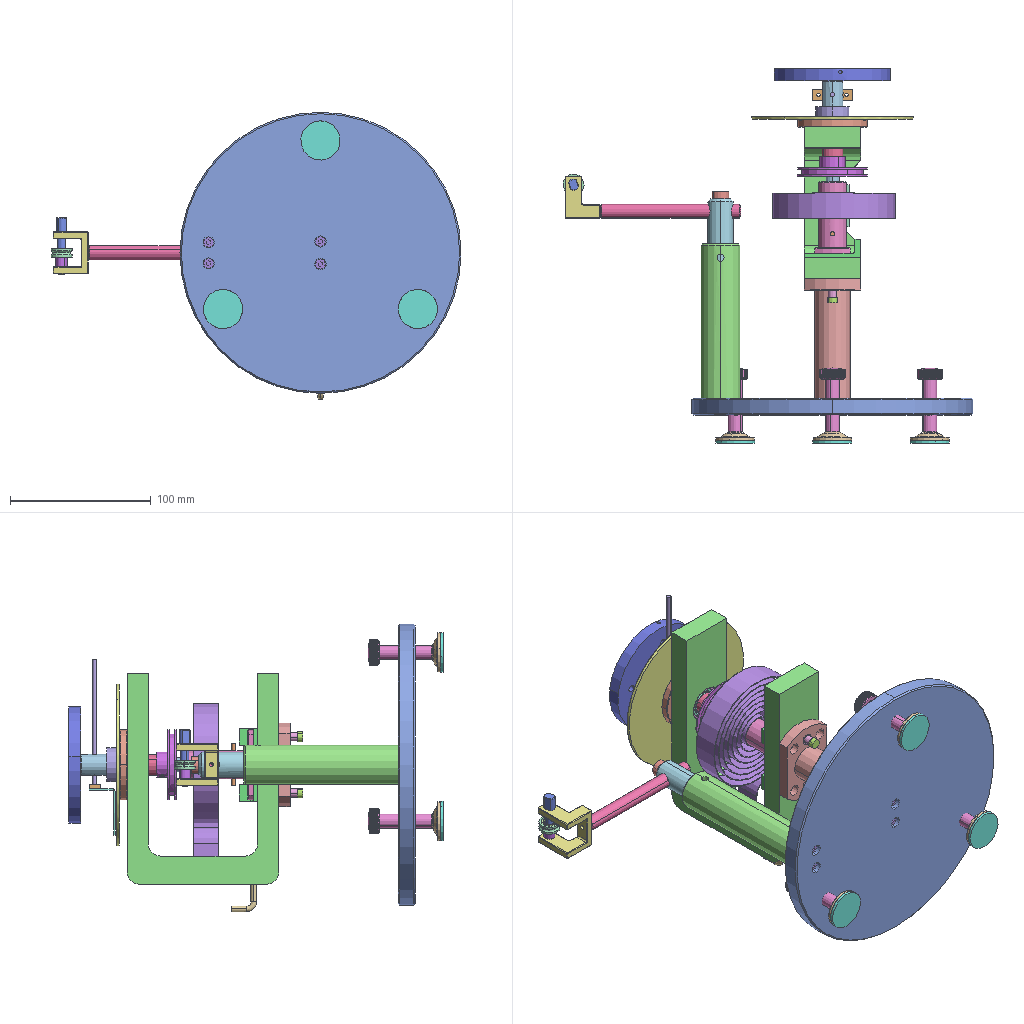Assembly | SolidWorks | 53 different items | 72 placed | box 292 x 266 x 204 mm
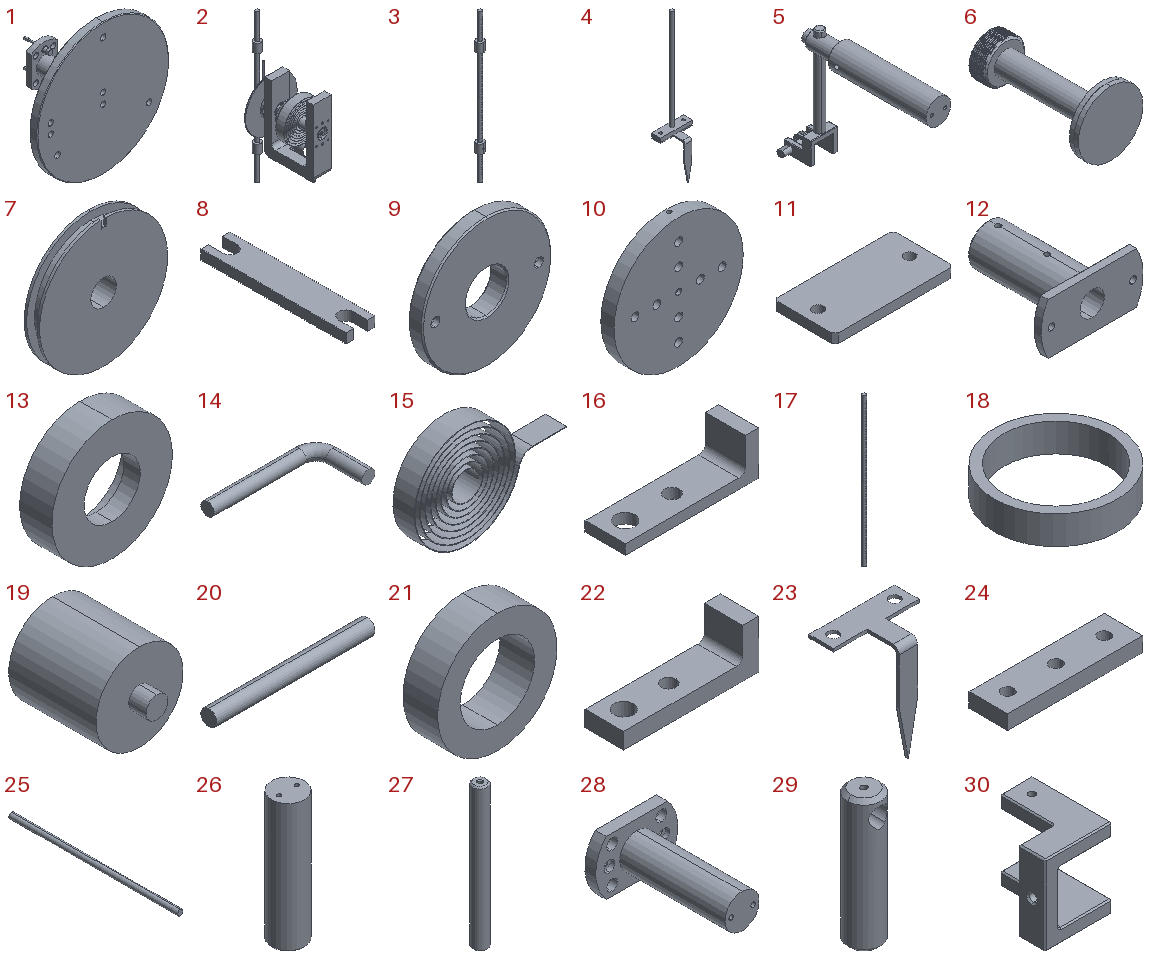Parts list (item | name | quantity | parent item | size | volume | features):
1 | (subassembly) | x1 | - | 200 x 119 x 200 mm | 427513 mm3 | -
2 | (subassembly) | x1 | - | 115 x 153 x 330 mm | 328755 mm3 | features CompositeCurve 2
3 | (subassembly) | x1 | in 2 | 16 x 16 x 330 mm | 22461 mm3 | features MirrorCompFeat 1, ReferencePattern 1
4 | (subassembly) | x1 | in 2 | 28 x 18.5 x 125 mm | 1686 mm3 | -
5 | (subassembly) | x1 | - | 40.5 x 159.5 x 126.5 mm | 84621 mm3 | -
6 | (subassembly) | x3 | - | 28 x 53.48 x 28 mm | 7166 mm3 | -
7 | - | x1 | in 2 | 50 x 14 x 50 mm | 10920 mm3 | features 3DProfileFeature 1, HoleWzd 1, ICE 1, Revolution 1
8 | - | x1 | in 2 | 6 x 30 x 2 mm | 309.863 mm3 | features Extrusion 1
9 | - | x1 | in 2 | 50 x 7 x 50 mm | 9665 mm3 | features 3DProfileFeature 1, Chamfer 1, HoleWzd 1, Revolution 1
10 | - | x1 | in 2 | 83 x 8.5 x 83 mm | 20251 mm3 | features 3DProfileFeature 1, Chamfer 1, HoleWzd 1, ICE 1, Revolution 1
11 | - | x1 | in 2 | 39 x 20 x 3 mm | 2276 mm3 | features Chamfer 1, Extrusion 1
12 | - | x1 | in 2 | 50 x 51 x 25 mm | 13586 mm3 | features 3DProfileFeature 2, HoleWzd 2, ICE 2, Chamfer 1, Revolution 1
13 | - | x1 | in 2 | 15 x 4 x 15 mm | 456.709 mm3 | features Revolution 1
14 | - | x1 | in 2 | 35 x 18 x 4 mm | 588.784 mm3 | features Sweep 1
15 | - | x1 | in 2 | 128.799 x 18 x 87.599 mm | 12839 mm3 | features Helix 1, Sweep 1
16 | - | x2 | in 2 | 40 x 12 x 13 mm | 1798 mm3 | features Extrusion 1, Fillet 1, ICE 1
17 | - | x1 | in 3 | 8 x 8 x 330 mm | 16519 mm3 | features ICE 3, LPattern 2, Extrusion 1
18 | - | x1 | in 2 | 26 x 26 x 6 mm | 904.779 mm3 | features Extrusion 1
19 | - | x2 | in 2 | 20 x 24 x 20 mm | 6362 mm3 | features Revolution 1
20 | - | x1 | in 2 | 30 x 3 x 3 mm | 212.058 mm3 | features Revolution 1
21 | - | x1 | in 2 | 24 x 7 x 24 mm | 1930 mm3 | features Extrusion 1
22 | - | x1 | in 2 | 42 x 12 x 15 mm | 2909 mm3 | features Extrusion 1, Fillet 1, ICE 1
23 | - | x1 | in 4 | 28 x 18.5 x 33 mm | 407.895 mm3 | features EdgeFlange 1, FlatPattern 1, SMBaseFlange 1, SheetMetal 1
24 | - | x1 | in 4 | 28 x 8 x 3 mm | 627.821 mm3 | features 3DProfileFeature 2, HoleWzd 2, Extrusion 1
25 | - | x1 | in 4 | 3 x 92 x 3 mm | 650.31 mm3 | features Revolution 1
26 | - | x1 | in 5 | 28 x 28 x 110 mm | 51946 mm3 | features 3DProfileFeature 2, HoleWzd 2, Chamfer 1, Revolution 1
27 | - | x1 | in 5 | 10 x 10 x 100 mm | 7790 mm3 | features Chamfer 2, Extrusion 1, HoleWzd 1
28 | - | x1 | in 1 | 60 x 85 x 40 mm | 53675 mm3 | features 3DProfileFeature 4, HoleWzd 4, ICE 1, Revolution 1
29 | - | x1 | in 5 | 18 x 18 x 72 mm | 16626 mm3 | features Chamfer 1, Extrusion 1, HoleWzd 1, ICE 1
30 | - | x1 | in 5 | 25 x 30 x 30 mm | 5700 mm3 | features Chamfer 3, ICE 3, 3DProfileFeature 1, Extrusion 1, Fillet 1, HoleWzd 1
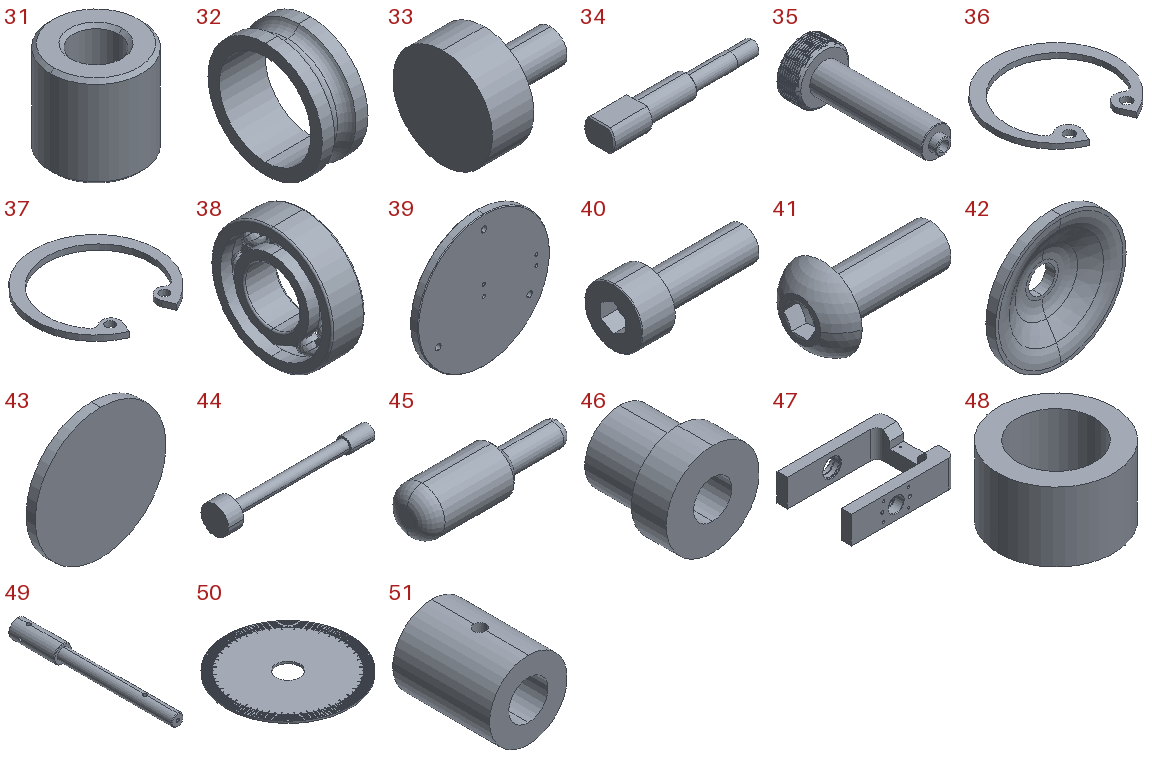31 | - | x1 | in 5 | 8 x 8 x 8 mm | 298.2 mm3 | features Chamfer 1, Extrusion 1
32 | - | x1 | in 5 | 6 x 15 x 15 mm | 290.652 mm3 | features Revolution 1
33 | - | x1 | in 5 | 13 x 12 x 12 mm | 666.018 mm3 | features Revolution 1
34 | - | x1 | in 5 | 40.5 x 8 x 6 mm | 1008 mm3 | features Chamfer 1, ICE 1, Revolution 1
35 | - | x3 | in 6 | 18 x 48 x 18 mm | 4770 mm3 | features Helix 2, SweepCut 2, Chamfer 1, CirPattern 1, HoleWzd 1, Revolution 1
36 | - | x1 | in 2 | 23.5 x 22.606 x 1 mm | 131.088 mm3 | features Extrusion 1
37 | - | x2 | in 2 | 26.9 x 25.876 x 1.2 mm | 193.596 mm3 | features Extrusion 1
38 | - | x2 | in 2 | 6 x 22 x 22 mm | 1184 mm3 | features Revolution 5, CirPattern 2, RevCut 2
39 | - | x1 | in 1 | 200 x 12 x 200 mm | 372597 mm3 | features 3DProfileFeature 2, HoleWzd 2, Chamfer 1, Extrusion 1
40 | - | x4 | - | 16 x 7 x 7 mm | 288.227 mm3 | features BlendCut 1, Cut 1, Fillet 1, LPattern 1, RevCut 1, Revolution 1
41 | - | x2 | in 2 | 9.65 x 5.7 x 5.7 mm | 80.901 mm3 | features RevCut 2, Revolution 2, Cut 1, LPattern 1, RefAxis 1
42 | - | x3 | in 6 | 27.8 x 5.98 x 27.8 mm | 1165 mm3 | features Revolution 1
43 | - | x3 | in 6 | 28 x 2 x 28 mm | 1232 mm3 | features Extrusion 1
44 | - | x2 | in 1 | 38.91 x 7 x 7 mm | 397.089 mm3 | features Revolution 1
45 | - | x1 | - | 20 x 6 x 6 mm | 371.971 mm3 | features Fillet 2, Chamfer 1, Revolution 1
46 | - | x2 | in 1 | 8 x 8 x 8 mm | 223.744 mm3 | features 3DProfileFeature 1, HoleWzd 1, Revolution 1
47 | - | x1 | in 2 | 150 x 108 x 40 mm | 209243 mm3 | features ICE 6, 3DProfileFeature 4, HoleWzd 4, Chamfer 1, Extrusion 1, LPattern 1
48 | - | x1 | in 2 | 15 x 15 x 9 mm | 883.573 mm3 | features Extrusion 1
49 | - | x1 | in 2 | 15 x 136.5 x 15 mm | 14219 mm3 | features 3DProfileFeature 3, HoleWzd 3, ICE 2, Chamfer 1, Revolution 1
50 | - | x1 | in 2 | 115 x 115 x 2 mm | 19943 mm3 | features ICE 2, CirPattern 1, Extrusion 1
51 | - | x2 | in 3 | 16 x 20 x 16 mm | 2971 mm3 | features 3DProfileFeature 1, HoleWzd 1, Revolution 1
52 | angular contact ball bearings gb | x1 | - | - | - | -
53 | deep groove ball bearings gb | x1 | - | - | - | -
Mates (type | each side: item.copy, entity, surface, feature):
In the top assembly
Coincident | 40.1 face plane Base-Revolve | 40.2 face plane Base-Revolve
Coincident | 40.3 face plane Base-Revolve | 40.4 face plane Base-Revolve
Coincident | 40.1 face plane Base-Revolve | 40.3 face plane Base-Revolve
Coincident | 39.1 face plane Boss-Extrude1 | assembly plane
Coincident | 39.1 plane | assembly plane
Concentric | 39.1 face cylinder M10 Tapped Hole1 | 35.1 face cylinder Revolve1
DistanceDim | 43.1 face plane Boss-Extrude1 | 39.1 face plane Boss-Extrude1
Concentric | 39.1 face cylinder CBORE for M4 Hex Head Bolt1 | 40.1 face cylinder Base-Revolve
Concentric | 39.1 face cylinder CBORE for M4 Hex Head Bolt1 | 40.4 face cylinder Base-Revolve
Concentric | 39.1 face cylinder CBORE for M4 Hex Head Bolt1 | 40.3 face cylinder Base-Revolve
Concentric | 39.1 face cylinder CBORE for M4 Hex Head Bolt1 | 40.2 face cylinder Base-Revolve
Coincident | 39.1 face plane CBORE for M4 Hex Head Bolt1 | 40.1 face plane Base-Revolve
Concentric | 47.1 face cylinder Cut-Extrude1 | 28.1 face cylinder Revolve1
Coincident | 47.1 face plane Boss-Extrude1 | 28.1 face plane Revolve1
Parallel | 47.1 face plane Boss-Extrude1 | 28.1 face plane Cut-Extrude2
Concentric | 26.1 face cylinder M4 Tapped Hole1 | 39.1 face cylinder CBORE for M4 Hex Head Bolt1 | 2 times
Coincident | 39.1 face plane Boss-Extrude1 | 26.1 face plane Revolve1
Concentric | 12.1 face cylinder M4 Tapped Hole1 | 44.1 face cylinder Revolve1
Coincident | 12.1 face plane Revolve1 | 44.1 face plane Revolve1
In subassembly 6
Coincident | 43.2 face plane Boss-Extrude1 | 42.1 face plane Revolve1
Concentric | 43.2 face cylinder Boss-Extrude1 | 42.1 face cylinder Revolve1
Concentric | 35.2 face cylinder Revolve1 | 42.1 face cylinder Revolve1
Coincident | 35.2 face plane Revolve1 | 42.1 face plane Revolve1
In subassembly 2
Concentric | 47.2 face cylinder Cut-Extrude1 | 49.1 face cylinder Revolve1
Concentric | 47.2 face cylinder Cut-Extrude2 | 9.1 face cylinder Revolve1
Coincident | 47.2 face plane Boss-Extrude1 | 9.1 face plane Revolve1
Concentric | 50.1 face cylinder Boss-Extrude1 | 9.1 face cylinder Revolve1
Coincident | 50.1 face plane Boss-Extrude1 | 9.1 face plane Revolve1
Concentric | 49.1 face cylinder Revolve1 | 38.1 face cylinder Boss-Revolve4
Concentric | 38.1 face cylinder Boss-Revolve3 | 18.1 face cylinder Boss-Extrude1
Concentric | 49.1 face cylinder Revolve1 | 7.1 face cylinder Revolve1
Coincident | 47.2 face plane Cut-Extrude5 | 11.1 face plane Boss-Extrude1
Concentric | 47.2 face cylinder M3 Tapped Hole2 | 11.1 face cylinder Boss-Extrude1 | 2 times
Coincident | 49.1 face plane Revolve1 | 38.1 face plane Boss-Revolve4
Concentric | 49.1 face cylinder Revolve1 | 12.2 face cylinder Revolve1
Parallel | 47.2 face plane Boss-Extrude1 | 12.2 face plane Cut-Extrude3
Concentric | 47.2 face cylinder LPattern1 | 37.1 face cylinder Base-Extrude
Coincident | 47.2 face plane LPattern1 | 37.1 face plane Base-Extrude
Concentric | 47.2 face cylinder Cut-Extrude3 | 36.1 face cylinder Base-Extrude
Concentric | 47.2 face cylinder Cut-Extrude4 | 37.2 face cylinder Base-Extrude
Coincident | 47.2 face plane Cut-Extrude4 | 37.2 face plane Base-Extrude
Concentric | 49.1 face cylinder Revolve1 | 38.2 face cylinder Boss-Revolve3
Coincident | 49.1 face plane Revolve1 | 10.1 face plane Revolve1
Concentric | 49.1 face cylinder Revolve1 | 10.1 face cylinder Revolve1
Coincident | 10.1 face plane Revolve1 | 19.1 face plane Revolve1
Concentric | 10.1 face cylinder Cut-Extrude1 | 19.1 face cylinder Revolve1
Concentric | 10.1 face cylinder Cut-Extrude1 | 19.2 face cylinder Revolve1
Coincident | 10.1 face plane Revolve1 | 19.2 face plane Revolve1
Concentric | 49.1 face cylinder Revolve1 | 48.1 face cylinder Boss-Extrude1
Coincident | 7.1 face plane Revolve1 | 48.1 face plane Boss-Extrude1
Concentric | 17.1 face cylinder Cut-Extrude1 | 49.1 face cylinder M4 Tapped Hole1
Concentric | 25.1 face cylinder Revolve1 | 49.1 face cylinder Cut-Extrude1
Parallel | 50.1 face plane Boss-Extrude1 | 23.1 face plane Edge-Flange1
Coincident | 47.2 face plane Cut-Extrude3 | 36.1 face plane Base-Extrude
Concentric | 49.1 face cylinder Revolve1 | 13.1 face cylinder Revolve1
Coincident | 13.1 face plane Revolve1 | 38.2 face plane Boss-Revolve4
Coincident | 47.2 face plane Cut-Extrude3 | 38.2 face plane Boss-Revolve3
DistanceDim | 25.1 face plane Revolve1 | 47.2 face plane Boss-Extrude1
Concentric | 12.2 face cylinder Revolve1 | 15.1 select_type:24
Parallel | 47.2 face plane Cut-Extrude5 | 15.1 face plane Sweep1
Concentric | 47.2 face cylinder M4 Tapped Hole1 | 14.1 face cylinder Sweep1
Parallel | 47.2 face plane Boss-Extrude1 | 14.1 face plane Sweep1
Coincident | 47.2 edge | 14.1 face plane Sweep1
Concentric | 8.1 face cylinder Boss-Extrude1 | 12.2 face cylinder M3 Tapped Hole1 | 3 times
Tangent | 8.1 face plane Boss-Extrude1 | 12.2 face cylinder Revolve1
Width | 15.1 face plane Sweep1 | 15.1 face plane Sweep1 | 8.1 face plane Boss-Extrude1 | 8.1 face plane Boss-Extrude1
Coincident | 47.2 face plane Boss-Extrude1 | 16.1 face plane Boss-Extrude1
Concentric | 12.2 face cylinder M4 Tapped Hole1 | 16.1 face cylinder Boss-Extrude1
Coincident | 12.2 face plane Revolve1 | 16.1 face plane Boss-Extrude1
Parallel | 47.2 face plane Boss-Extrude1 | 16.1 face plane Boss-Extrude1
Concentric | 12.2 face cylinder M4 Tapped Hole1 | 16.2 face cylinder Boss-Extrude1
Coincident | 47.2 face plane Boss-Extrude1 | 16.2 face plane Boss-Extrude1
Parallel | 47.2 face plane Boss-Extrude1 | 16.2 face plane Boss-Extrude1
Concentric | 47.2 face cylinder M3 Tapped Hole2 | 41.1 face cylinder Revolve1
Coincident | 11.1 face plane Boss-Extrude1 | 41.1 face plane Revolve1
Concentric | 11.1 face cylinder Boss-Extrude1 | 41.2 face cylinder Revolve1
Coincident | 11.1 face plane Boss-Extrude1 | 41.2 face plane Revolve1
Coincident | 47.2 plane | 2.1 plane
Coincident | 47.2 face plane LPattern1 | 18.1 face plane Boss-Extrude1
Coincident | 18.1 face plane Boss-Extrude1 | 38.1 face plane Boss-Revolve3
Coincident | 48.1 face plane Boss-Extrude1 | 38.1 face plane Boss-Revolve4
Concentric | 49.1 face cylinder Cut-Extrude2 | 20.1 face cylinder Revolve1
Tangent | 49.1 face plane Revolve1 | 17.1 face cylinder Boss-Extrude1
Concentric | 47.2 face cylinder M3 Tapped Hole1 | 9.1 face cylinder CBORE for M3 Hex Head Bolt1
Parallel | 23.1 face plane Base-Flange1 | 51.1 face plane Revolve1
Concentric | 49.1 face cylinder Revolve1 | 21.1 face cylinder Boss-Extrude1
Coincident | 50.1 face plane Boss-Extrude1 | 21.1 face plane Boss-Extrude1
Parallel | 23.1 face plane Base-Flange1 | 47.2 face plane Boss-Extrude1
Concentric | 12.2 face cylinder M4 Tapped Hole1 | 22.1 face
Parallel | 47.2 face plane Boss-Extrude1 | 22.1 face
Coincident | 47.2 face plane Boss-Extrude1 | 22.1 face
In subassembly 3
Concentric | 51.2 face cylinder Revolve1 | 17.2 face cylinder Boss-Extrude1
In subassembly 4
Concentric | 24.1 face cylinder M3 Tapped Hole1 | 25.2 face cylinder Revolve1
Concentric | 23.2 face cylinder Base-Flange1 | 24.1 face cylinder Boss-Extrude1 | 2 times
Coincident | 23.2 face plane Base-Flange1 | 24.1 face plane Boss-Extrude1
Coincident | 23.2 face plane Base-Flange1 | 25.2 face plane Revolve1
In subassembly 1
Coincident | 39.2 face plane Boss-Extrude1 | 28.2 face plane Revolve1
Concentric | 39.2 face cylinder CBORE for M4 Hex Head Bolt1 | 28.2 face cylinder M4 Tapped Hole1 | 2 times
Concentric | 28.2 face cylinder CBORE for M4 Hex Head Bolt1 | 46.1 face cylinder Revolve1
Coincident | 28.2 face plane CBORE for M4 Hex Head Bolt1 | 46.1 face plane Revolve1
Concentric | 46.2 face cylinder Revolve1 | 44.2 face cylinder Revolve1
Coincident | 46.2 face plane Revolve1 | 44.2 face plane Revolve1 | 2 times
Coincident | 28.2 face plane CBORE for M4 Hex Head Bolt1 | 46.2 face plane Revolve1
Concentric | 28.2 face cylinder M4 Tapped Hole4 | 44.2 face cylinder Revolve1
Coincident | 39.2 plane | 1.1 plane
Concentric | 44.3 face cylinder Revolve1 | 46.1 face cylinder Revolve1
Coincident | 44.3 face plane Revolve1 | 46.1 face plane Revolve1
In subassembly 5
Coincident | 26.2 face plane Revolve1 | 5.1 plane
Coincident | 26.2 plane | 5.1 plane | 2 times
Concentric | 26.2 face cylinder Revolve1 | 29.1 face cylinder Boss-Extrude1
DistanceDim | 29.1 face plane Boss-Extrude1 | 26.2 face plane Revolve1
Concentric | 27.1 face cylinder Boss-Extrude1 | 29.1 face cylinder Cut-Extrude1
Concentric | 27.1 face cylinder M3 Tapped Hole1 | 30.1 face cylinder Cut-Extrude2
Coincident | 27.1 face plane Boss-Extrude1 | 30.1 face plane Boss-Extrude1
Parallel | 26.2 face plane Revolve1 | 30.1 face plane Boss-Extrude1
Concentric | 29.1 face cylinder M4 Tapped Hole1 | 33.1 face cylinder Revolve1
Coincident | 29.1 face plane Boss-Extrude1 | 33.1 face plane Revolve1
Concentric | 30.1 face cylinder Cut-Extrude5 | 31.1 face cylinder Boss-Extrude1
Width | 32.1 face plane Revolve1 | 32.1 face plane Revolve1 | 30.1 face plane Boss-Extrude1 | 30.1 face plane Boss-Extrude1
Coincident | 30.1 face plane Boss-Extrude1 | 34.1 face plane Revolve1
Parallel | 26.2 plane | 30.1 face plane Boss-Extrude1